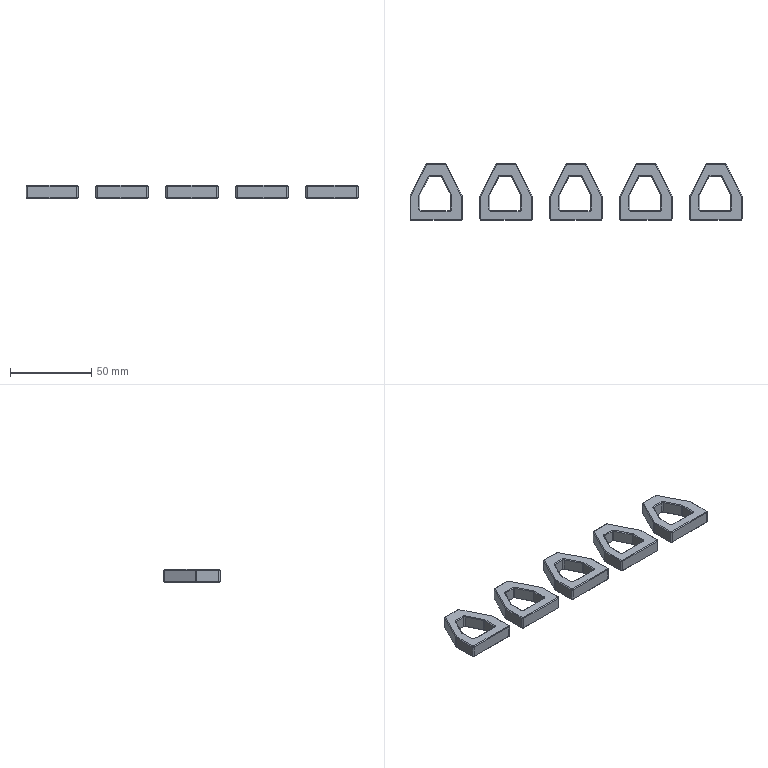NC program | NX | posted with a generic post | part box 204 x 35 x 8 mm
Lines 3701 to 4636 of 15564:
(ZLEVEL_PROFILE_COPY_1_COPY_1 , TOOL : D4)
N7382 T11 M6
N7384 G54
N7386 G17 G0 G90 X90.756 Y-9.215 S9500 M3
N7388 G43 Z30. H11
N7390 Z-0.385
N7392 G94 G1 X90.872 Y-9.415 F1000.
N7394 G3 X91.218 Y-9.615 R0.4
N7396 G1 X94.115 F1800.
N7398 Y-6.718
N7400 G3 X93.915 Y-6.372 R0.4
N7402 G1 X93.715 Y-6.256
N7404 G0 X90.641 Y-9.1 Z-0.769
N7406 G1 X90.757 Y-9.3 F1000.
N7408 G3 X91.103 Y-9.5 R0.4
N7410 G1 X94. F1800.
N7412 Y-6.603
N7414 G3 X93.8 Y-6.257 R0.4
N7416 G1 X93.6 Y-6.141
N7418 G0 X90.641 Y-9.1 Z-1.154
N7420 G1 X90.757 Y-9.3 F1000.
N7422 G3 X91.103 Y-9.5 R0.4
N7424 G1 X94. F1800.
N7426 Y-6.603
N7428 G3 X93.8 Y-6.257 R0.4
N7430 G1 X93.6 Y-6.141
N7432 G0 X90.641 Y-9.1 Z-1.538
N7434 G1 X90.757 Y-9.3 F1000.
N7436 G3 X91.103 Y-9.5 R0.4
N7438 G1 X94. F1800.
N7440 Y-6.603
N7442 G3 X93.8 Y-6.257 R0.4
N7444 G1 X93.6 Y-6.141
N7446 G0 X90.641 Y-9.1 Z-1.923
N7448 G1 X90.757 Y-9.3 F1000.
N7450 G3 X91.103 Y-9.5 R0.4
N7452 G1 X94. F1800.
N7454 Y-6.603
N7456 G3 X93.8 Y-6.257 R0.4
N7458 G1 X93.6 Y-6.141
N7460 G0 X90.641 Y-9.1 Z-2.308
N7462 G1 X90.757 Y-9.3 F1000.
N7464 G3 X91.103 Y-9.5 R0.4
N7466 G1 X94. F1800.
N7468 Y-6.603
N7470 G3 X93.8 Y-6.257 R0.4
N7472 G1 X93.6 Y-6.141
N7474 G0 X90.641 Y-9.1 Z-2.692
N7476 G1 X90.757 Y-9.3 F1000.
N7478 G3 X91.103 Y-9.5 R0.4
N7480 G1 X94. F1800.
N7482 Y-6.603
N7484 G3 X93.8 Y-6.257 R0.4
N7486 G1 X93.6 Y-6.141
N7488 G0 X90.641 Y-9.1 Z-3.077
N7490 G1 X90.757 Y-9.3 F1000.
N7492 G3 X91.103 Y-9.5 R0.4
N7494 G1 X94. F1800.
N7496 Y-6.603
N7498 G3 X93.8 Y-6.257 R0.4
N7500 G1 X93.6 Y-6.141
N7502 G0 X90.641 Y-9.1 Z-3.462
N7504 G1 X90.757 Y-9.3 F1000.
N7506 G3 X91.103 Y-9.5 R0.4
N7508 G1 X94. F1800.
N7510 Y-6.603
N7512 G3 X93.8 Y-6.257 R0.4
N7514 G1 X93.6 Y-6.141
N7516 G0 X90.641 Y-9.1 Z-3.846
N7518 G1 X90.757 Y-9.3 F1000.
N7520 G3 X91.103 Y-9.5 R0.4
N7522 G1 X94. F1800.
N7524 Y-6.603
N7526 G3 X93.8 Y-6.257 R0.4
N7528 G1 X93.6 Y-6.141
N7530 G0 X90.641 Y-9.1 Z-4.231
N7532 G1 X90.757 Y-9.3 F1000.
N7534 G3 X91.103 Y-9.5 R0.4
N7536 G1 X94. F1800.
N7538 Y-6.603
N7540 G3 X93.8 Y-6.257 R0.4
N7542 G1 X93.6 Y-6.141
N7544 G0 X90.641 Y-9.1 Z-4.615
N7546 G1 X90.757 Y-9.3 F1000.
N7548 G3 X91.103 Y-9.5 R0.4
N7550 G1 X94. F1800.
N7552 Y-6.603
N7554 G3 X93.8 Y-6.257 R0.4
N7556 G1 X93.6 Y-6.141
N7558 G0 X90.641 Y-9.1 Z-5.
N7560 G1 X90.757 Y-9.3 F1000.
N7562 G3 X91.103 Y-9.5 R0.4
N7564 G1 X94. F1800.
N7566 Y-6.603
N7568 G3 X93.8 Y-6.257 R0.4
N7570 G1 X93.6 Y-6.141
N7572 G0 X90.641 Y-9.1 Z-5.333
N7574 G1 X90.757 Y-9.3 F1000.
N7576 G3 X91.103 Y-9.5 R0.4
N7578 G1 X94. F1800.
N7580 Y-6.603
N7582 G3 X93.8 Y-6.257 R0.4
N7584 G1 X93.6 Y-6.141
N7586 G0 X90.641 Y-9.1 Z-5.667
N7588 G1 X90.757 Y-9.3 F1000.
N7590 G3 X91.103 Y-9.5 R0.4
N7592 G1 X94. F1800.
N7594 Y-6.603
N7596 G3 X93.8 Y-6.257 R0.4
N7598 G1 X93.6 Y-6.141
N7600 G0 X90.641 Y-9.1 Z-6.
N7602 G1 X90.757 Y-9.3 F1000.
N7604 G3 X91.103 Y-9.5 R0.4
N7606 G1 X94. F1800.
N7608 Y-6.603
N7610 G3 X93.8 Y-6.257 R0.4
N7612 G1 X93.6 Y-6.141
N7614 G0 X90.641 Y-9.1 Z-6.4
N7616 G1 X90.757 Y-9.3 F1000.
N7618 G3 X91.103 Y-9.5 R0.4
N7620 G1 X94. F1800.
N7622 Y-6.603
N7624 G3 X93.8 Y-6.257 R0.4
N7626 G1 X93.6 Y-6.141
N7628 G0 X90.641 Y-9.1 Z-6.8
N7630 G1 X90.757 Y-9.3 F1000.
N7632 G3 X91.103 Y-9.5 R0.4
N7634 G1 X94. F1800.
N7636 Y-6.603
N7638 G3 X93.8 Y-6.257 R0.4
N7640 G1 X93.6 Y-6.141
N7642 G0 X90.641 Y-9.1 Z-7.2
N7644 G1 X90.757 Y-9.3 F1000.
N7646 G3 X91.103 Y-9.5 R0.4
N7648 G1 X94. F1800.
N7650 Y-6.603
N7652 G3 X93.8 Y-6.257 R0.4
N7654 G1 X93.6 Y-6.141
N7656 G0 X90.641 Y-9.1 Z-7.6
N7658 G1 X90.757 Y-9.3 F1000.
N7660 G3 X91.103 Y-9.5 R0.4
N7662 G1 X94. F1800.
N7664 Y-6.603
N7666 G3 X93.8 Y-6.257 R0.4
N7668 G1 X93.6 Y-6.141
N7670 G0 X90.641 Y-9.1 Z-8.
N7672 G1 X90.757 Y-9.3 F1000.
N7674 G3 X91.103 Y-9.5 R0.4
N7676 G1 X94. F1800.
N7678 Y-6.603
N7680 G3 X93.8 Y-6.257 R0.4
N7682 G1 X93.6 Y-6.141
N7684 G0 Z30.
N7686 X93.715 Y-3.428
N7688 Z-0.385
N7690 G1 X93.915 Y-3.313 F1000.
N7692 G3 X94.115 Y-2.967 R0.4
N7694 G1 Y-2.361 F1800.
N7696 X93.845 Y-1.82
N7698 G3 X93.511 Y-1.6 R0.4
N7700 G1 X93.28 Y-1.586
N7702 G0 X93.6 Y-3.456 Z-0.769
N7704 G1 X93.8 Y-3.34 F1000.
N7706 G3 X94. Y-2.994 R0.4
N7708 G1 Y-2.389 F1800.
N7710 X93.729 Y-1.847
N7712 G3 X93.396 Y-1.627 R0.4
N7714 G1 X93.165 Y-1.613
N7716 G0 X93.6 Y-3.456 Z-1.154
N7718 G1 X93.8 Y-3.34 F1000.
N7720 G3 X94. Y-2.994 R0.4
N7722 G1 Y-2.389 F1800.
N7724 X93.729 Y-1.847
N7726 G3 X93.396 Y-1.627 R0.4
N7728 G1 X93.165 Y-1.613
N7730 G0 X93.6 Y-3.456 Z-1.538
N7732 G1 X93.8 Y-3.34 F1000.
N7734 G3 X94. Y-2.994 R0.4
N7736 G1 Y-2.389 F1800.
N7738 X93.729 Y-1.847
N7740 G3 X93.396 Y-1.627 R0.4
N7742 G1 X93.165 Y-1.613
N7744 G0 X93.6 Y-3.456 Z-1.923
N7746 G1 X93.8 Y-3.34 F1000.
N7748 G3 X94. Y-2.994 R0.4
N7750 G1 Y-2.389 F1800.
N7752 X93.729 Y-1.847
N7754 G3 X93.396 Y-1.627 R0.4
N7756 G1 X93.165 Y-1.613
N7758 G0 X93.6 Y-3.456 Z-2.308
N7760 G1 X93.8 Y-3.34 F1000.
N7762 G3 X94. Y-2.994 R0.4
N7764 G1 Y-2.389 F1800.
N7766 X93.729 Y-1.847
N7768 G3 X93.396 Y-1.627 R0.4
N7770 G1 X93.165 Y-1.613
N7772 G0 X93.6 Y-3.456 Z-2.692
N7774 G1 X93.8 Y-3.34 F1000.
N7776 G3 X94. Y-2.994 R0.4
N7778 G1 Y-2.389 F1800.
N7780 X93.729 Y-1.847
N7782 G3 X93.396 Y-1.627 R0.4
N7784 G1 X93.165 Y-1.613
N7786 G0 X93.6 Y-3.456 Z-3.077
N7788 G1 X93.8 Y-3.34 F1000.
N7790 G3 X94. Y-2.994 R0.4
N7792 G1 Y-2.389 F1800.
N7794 X93.729 Y-1.847
N7796 G3 X93.396 Y-1.627 R0.4
N7798 G1 X93.165 Y-1.613
N7800 G0 X93.6 Y-3.456 Z-3.462
N7802 G1 X93.8 Y-3.34 F1000.
N7804 G3 X94. Y-2.994 R0.4
N7806 G1 Y-2.389 F1800.
N7808 X93.729 Y-1.847
N7810 G3 X93.396 Y-1.627 R0.4
N7812 G1 X93.165 Y-1.613
N7814 G0 X93.6 Y-3.456 Z-3.846
N7816 G1 X93.8 Y-3.34 F1000.
N7818 G3 X94. Y-2.994 R0.4
N7820 G1 Y-2.389 F1800.
N7822 X93.729 Y-1.847
N7824 G3 X93.396 Y-1.627 R0.4
N7826 G1 X93.165 Y-1.613
N7828 G0 X93.6 Y-3.456 Z-4.231
N7830 G1 X93.8 Y-3.34 F1000.
N7832 G3 X94. Y-2.994 R0.4
N7834 G1 Y-2.389 F1800.
N7836 X93.729 Y-1.847
N7838 G3 X93.396 Y-1.627 R0.4
N7840 G1 X93.165 Y-1.613
N7842 G0 X93.6 Y-3.456 Z-4.615
N7844 G1 X93.8 Y-3.34 F1000.
N7846 G3 X94. Y-2.994 R0.4
N7848 G1 Y-2.389 F1800.
N7850 X93.729 Y-1.847
N7852 G3 X93.396 Y-1.627 R0.4
N7854 G1 X93.165 Y-1.613
N7856 G0 X93.6 Y-3.456 Z-5.
N7858 G1 X93.8 Y-3.34 F1000.
N7860 G3 X94. Y-2.994 R0.4
N7862 G1 Y-2.389 F1800.
N7864 X93.729 Y-1.847
N7866 G3 X93.396 Y-1.627 R0.4
N7868 G1 X93.165 Y-1.613
N7870 G0 X93.6 Y-3.456 Z-5.333
N7872 G1 X93.8 Y-3.34 F1000.
N7874 G3 X94. Y-2.994 R0.4
N7876 G1 Y-2.389 F1800.
N7878 X93.729 Y-1.847
N7880 G3 X93.396 Y-1.627 R0.4
N7882 G1 X93.165 Y-1.613
N7884 G0 X93.6 Y-3.456 Z-5.667
N7886 G1 X93.8 Y-3.34 F1000.
N7888 G3 X94. Y-2.994 R0.4
N7890 G1 Y-2.389 F1800.
N7892 X93.729 Y-1.847
N7894 G3 X93.396 Y-1.627 R0.4
N7896 G1 X93.165 Y-1.613
N7898 G0 X93.6 Y-3.456 Z-6.
N7900 G1 X93.8 Y-3.34 F1000.
N7902 G3 X94. Y-2.994 R0.4
N7904 G1 Y-2.389 F1800.
N7906 X93.729 Y-1.847
N7908 G3 X93.396 Y-1.627 R0.4
N7910 G1 X93.165 Y-1.613
N7912 G0 X93.6 Y-3.456 Z-6.4
N7914 G1 X93.8 Y-3.34 F1000.
N7916 G3 X94. Y-2.994 R0.4
N7918 G1 Y-2.389 F1800.
N7920 X93.729 Y-1.847
N7922 G3 X93.396 Y-1.627 R0.4
N7924 G1 X93.165 Y-1.613
N7926 G0 X93.6 Y-3.456 Z-6.8
N7928 G1 X93.8 Y-3.34 F1000.
N7930 G3 X94. Y-2.994 R0.4
N7932 G1 Y-2.389 F1800.
N7934 X93.729 Y-1.847
N7936 G3 X93.396 Y-1.627 R0.4
N7938 G1 X93.165 Y-1.613
N7940 G0 X93.6 Y-3.456 Z-7.2
N7942 G1 X93.8 Y-3.34 F1000.
N7944 G3 X94. Y-2.994 R0.4
N7946 G1 Y-2.389 F1800.
N7948 X93.729 Y-1.847
N7950 G3 X93.396 Y-1.627 R0.4
N7952 G1 X93.165 Y-1.613
N7954 G0 X93.6 Y-3.454 Z-7.6
N7956 G1 X93.8 Y-3.339 F1000.
N7958 G3 X94. Y-2.993 R0.4
N7960 G1 Y-2.389 F1800.
N7962 X93.73 Y-1.848
N7964 G3 X93.396 Y-1.628 R0.4
N7966 G1 X93.165 Y-1.614
N7968 G0 X93.6 Y-3.454 Z-8.
N7970 G1 X93.8 Y-3.339 F1000.
N7972 G3 X94. Y-2.993 R0.4
N7974 G1 Y-2.389 F1800.
N7976 X93.73 Y-1.848
N7978 G3 X93.396 Y-1.628 R0.4
N7980 G1 X93.165 Y-1.614
N7982 G0 Z30.
N7984 X89.759 Y5.457
N7986 Z-0.385
N7988 G1 X89.886 Y5.65 F1000.
N7990 G3 X89.91 Y6.049 R0.4
N7992 G1 X89.127 Y7.615 F1800.
N7994 X87.376
N7996 G3 X87.03 Y7.415 R0.4
N7998 G1 X86.914 Y7.215
N8000 G0 X89.688 Y5.342 Z-0.769
N8002 G1 X89.815 Y5.534 F1000.
N8004 G3 X89.839 Y5.934 R0.4
N8006 G1 X89.056 Y7.5 F1800.
N8008 X87.305
N8010 G3 X86.958 Y7.3 R0.4
N8012 G1 X86.843 Y7.1
N8014 G0 X89.688 Y5.342 Z-1.154
N8016 G1 X89.815 Y5.534 F1000.
N8018 G3 X89.839 Y5.934 R0.4
N8020 G1 X89.056 Y7.5 F1800.
N8022 X87.305
N8024 G3 X86.958 Y7.3 R0.4
N8026 G1 X86.843 Y7.1
N8028 G0 X89.688 Y5.342 Z-1.538
N8030 G1 X89.815 Y5.534 F1000.
N8032 G3 X89.839 Y5.934 R0.4
N8034 G1 X89.056 Y7.5 F1800.
N8036 X87.305
N8038 G3 X86.958 Y7.3 R0.4
N8040 G1 X86.843 Y7.1
N8042 G0 X89.688 Y5.342 Z-1.923
N8044 G1 X89.815 Y5.534 F1000.
N8046 G3 X89.839 Y5.934 R0.4
N8048 G1 X89.056 Y7.5 F1800.
N8050 X87.305
N8052 G3 X86.958 Y7.3 R0.4
N8054 G1 X86.843 Y7.1
N8056 G0 X89.688 Y5.342 Z-2.308
N8058 G1 X89.815 Y5.534 F1000.
N8060 G3 X89.839 Y5.934 R0.4
N8062 G1 X89.056 Y7.5 F1800.
N8064 X87.305
N8066 G3 X86.958 Y7.3 R0.4
N8068 G1 X86.843 Y7.1
N8070 G0 X89.688 Y5.342 Z-2.692
N8072 G1 X89.815 Y5.534 F1000.
N8074 G3 X89.839 Y5.934 R0.4
N8076 G1 X89.056 Y7.5 F1800.
N8078 X87.305
N8080 G3 X86.958 Y7.3 R0.4
N8082 G1 X86.843 Y7.1
N8084 G0 X89.688 Y5.342 Z-3.077
N8086 G1 X89.815 Y5.534 F1000.
N8088 G3 X89.839 Y5.934 R0.4
N8090 G1 X89.056 Y7.5 F1800.
N8092 X87.305
N8094 G3 X86.958 Y7.3 R0.4
N8096 G1 X86.843 Y7.1
N8098 G0 X89.688 Y5.342 Z-3.462
N8100 G1 X89.815 Y5.534 F1000.
N8102 G3 X89.839 Y5.934 R0.4
N8104 G1 X89.056 Y7.5 F1800.
N8106 X87.305
N8108 G3 X86.958 Y7.3 R0.4
N8110 G1 X86.843 Y7.1
N8112 G0 X89.688 Y5.342 Z-3.846
N8114 G1 X89.815 Y5.534 F1000.
N8116 G3 X89.839 Y5.934 R0.4
N8118 G1 X89.056 Y7.5 F1800.
N8120 X87.305
N8122 G3 X86.958 Y7.3 R0.4
N8124 G1 X86.843 Y7.1
N8126 G0 X89.688 Y5.342 Z-4.231
N8128 G1 X89.815 Y5.534 F1000.
N8130 G3 X89.839 Y5.934 R0.4
N8132 G1 X89.056 Y7.5 F1800.
N8134 X87.305
N8136 G3 X86.958 Y7.3 R0.4
N8138 G1 X86.843 Y7.1
N8140 G0 X89.688 Y5.342 Z-4.615
N8142 G1 X89.815 Y5.534 F1000.
N8144 G3 X89.839 Y5.934 R0.4
N8146 G1 X89.056 Y7.5 F1800.
N8148 X87.305
N8150 G3 X86.958 Y7.3 R0.4
N8152 G1 X86.843 Y7.1
N8154 G0 X89.688 Y5.342 Z-5.
N8156 G1 X89.815 Y5.534 F1000.
N8158 G3 X89.839 Y5.934 R0.4
N8160 G1 X89.056 Y7.5 F1800.
N8162 X87.305
N8164 G3 X86.958 Y7.3 R0.4
N8166 G1 X86.843 Y7.1
N8168 G0 X89.688 Y5.342 Z-5.333
N8170 G1 X89.815 Y5.534 F1000.
N8172 G3 X89.839 Y5.934 R0.4
N8174 G1 X89.056 Y7.5 F1800.
N8176 X87.305
N8178 G3 X86.958 Y7.3 R0.4
N8180 G1 X86.843 Y7.1
N8182 G0 X89.688 Y5.342 Z-5.667
N8184 G1 X89.815 Y5.534 F1000.
N8186 G3 X89.839 Y5.934 R0.4
N8188 G1 X89.056 Y7.5 F1800.
N8190 X87.305
N8192 G3 X86.958 Y7.3 R0.4
N8194 G1 X86.843 Y7.1
N8196 G0 X89.688 Y5.342 Z-6.
N8198 G1 X89.815 Y5.534 F1000.
N8200 G3 X89.839 Y5.934 R0.4
N8202 G1 X89.056 Y7.5 F1800.
N8204 X87.305
N8206 G3 X86.958 Y7.3 R0.4
N8208 G1 X86.843 Y7.1
N8210 G0 X89.688 Y5.342 Z-6.4
N8212 G1 X89.815 Y5.534 F1000.
N8214 G3 X89.839 Y5.934 R0.4
N8216 G1 X89.056 Y7.5 F1800.
N8218 X87.305
N8220 G3 X86.958 Y7.3 R0.4
N8222 G1 X86.843 Y7.1
N8224 G0 X89.688 Y5.342 Z-6.8
N8226 G1 X89.815 Y5.534 F1000.
N8228 G3 X89.839 Y5.934 R0.4
N8230 G1 X89.056 Y7.5 F1800.
N8232 X87.305
N8234 G3 X86.958 Y7.3 R0.4
N8236 G1 X86.843 Y7.1
N8238 G0 X89.688 Y5.342 Z-7.2
N8240 G1 X89.815 Y5.534 F1000.
N8242 G3 X89.839 Y5.934 R0.4
N8244 G1 X89.056 Y7.5 F1800.
N8246 X87.305
N8248 G3 X86.958 Y7.3 R0.4
N8250 G1 X86.843 Y7.1
N8252 G0 X89.686 Y5.344 Z-7.6
N8254 G1 X89.814 Y5.537 F1000.
N8256 G3 X89.838 Y5.936 R0.4
N8258 G1 X89.056 Y7.5 F1800.
N8260 X87.307
N8262 G3 X86.96 Y7.3 R0.4
N8264 G1 X86.845 Y7.1
N8266 G0 X89.686 Y5.344 Z-8.
N8268 G1 X89.814 Y5.537 F1000.
N8270 G3 X89.838 Y5.936 R0.4
N8272 G1 X89.056 Y7.5 F1800.
N8274 X87.307
N8276 G3 X86.96 Y7.3 R0.4
N8278 G1 X86.845 Y7.1
N8280 G0 Z30.
N8282 X86.086 Y7.215
N8284 Z-0.385
N8286 G1 X85.97 Y7.415 F1000.
N8288 G3 X85.624 Y7.615 R0.4
N8290 G1 X83.873 F1800.
N8292 X83.09 Y6.049
N8294 G3 X83.114 Y5.65 R0.4
N8296 G1 X83.241 Y5.457
N8298 G0 X86.157 Y7.1 Z-0.769
N8300 G1 X86.042 Y7.3 F1000.
N8302 G3 X85.695 Y7.5 R0.4
N8304 G1 X83.944 F1800.
N8306 X83.161 Y5.934
N8308 G3 X83.185 Y5.535 R0.4
N8310 G1 X83.313 Y5.342
N8312 G0 X86.157 Y7.1 Z-1.154
N8314 G1 X86.042 Y7.3 F1000.
N8316 G3 X85.695 Y7.5 R0.4
N8318 G1 X83.944 F1800.
N8320 X83.161 Y5.934
N8322 G3 X83.185 Y5.535 R0.4
N8324 G1 X83.313 Y5.342
N8326 G0 X86.157 Y7.1 Z-1.538
N8328 G1 X86.042 Y7.3 F1000.
N8330 G3 X85.695 Y7.5 R0.4
N8332 G1 X83.944 F1800.
N8334 X83.161 Y5.934
N8336 G3 X83.185 Y5.535 R0.4
N8338 G1 X83.313 Y5.342
N8340 G0 X86.157 Y7.1 Z-1.923
N8342 G1 X86.042 Y7.3 F1000.
N8344 G3 X85.695 Y7.5 R0.4
N8346 G1 X83.944 F1800.
N8348 X83.161 Y5.934
N8350 G3 X83.185 Y5.535 R0.4
N8352 G1 X83.313 Y5.342
N8354 G0 X86.157 Y7.1 Z-2.308
N8356 G1 X86.042 Y7.3 F1000.
N8358 G3 X85.695 Y7.5 R0.4
N8360 G1 X83.944 F1800.
N8362 X83.161 Y5.934
N8364 G3 X83.185 Y5.535 R0.4
N8366 G1 X83.313 Y5.342
N8368 G0 X86.157 Y7.1 Z-2.692
N8370 G1 X86.042 Y7.3 F1000.
N8372 G3 X85.695 Y7.5 R0.4
N8374 G1 X83.944 F1800.
N8376 X83.161 Y5.934
N8378 G3 X83.185 Y5.535 R0.4
N8380 G1 X83.313 Y5.342
N8382 G0 X86.157 Y7.1 Z-3.077
N8384 G1 X86.042 Y7.3 F1000.
N8386 G3 X85.695 Y7.5 R0.4
N8388 G1 X83.944 F1800.
N8390 X83.161 Y5.934
N8392 G3 X83.185 Y5.535 R0.4
N8394 G1 X83.313 Y5.342
N8396 G0 X86.157 Y7.1 Z-3.462
N8398 G1 X86.042 Y7.3 F1000.
N8400 G3 X85.695 Y7.5 R0.4
N8402 G1 X83.944 F1800.
N8404 X83.161 Y5.934
N8406 G3 X83.185 Y5.535 R0.4
N8408 G1 X83.313 Y5.342
N8410 G0 X86.157 Y7.1 Z-3.846
N8412 G1 X86.042 Y7.3 F1000.
N8414 G3 X85.695 Y7.5 R0.4
N8416 G1 X83.944 F1800.
N8418 X83.161 Y5.934
N8420 G3 X83.185 Y5.535 R0.4
N8422 G1 X83.313 Y5.342
N8424 G0 X86.157 Y7.1 Z-4.231
N8426 G1 X86.042 Y7.3 F1000.
N8428 G3 X85.695 Y7.5 R0.4
N8430 G1 X83.944 F1800.
N8432 X83.161 Y5.934
N8434 G3 X83.185 Y5.535 R0.4
N8436 G1 X83.313 Y5.342
N8438 G0 X86.157 Y7.1 Z-4.615
N8440 G1 X86.042 Y7.3 F1000.
N8442 G3 X85.695 Y7.5 R0.4
N8444 G1 X83.944 F1800.
N8446 X83.161 Y5.934
N8448 G3 X83.185 Y5.535 R0.4
N8450 G1 X83.313 Y5.342
N8452 G0 X86.157 Y7.1 Z-5.
N8454 G1 X86.042 Y7.3 F1000.
N8456 G3 X85.695 Y7.5 R0.4
N8458 G1 X83.944 F1800.
N8460 X83.161 Y5.934
N8462 G3 X83.185 Y5.535 R0.4
N8464 G1 X83.313 Y5.342
N8466 G0 X86.157 Y7.1 Z-5.333
N8468 G1 X86.042 Y7.3 F1000.
N8470 G3 X85.695 Y7.5 R0.4
N8472 G1 X83.944 F1800.
N8474 X83.161 Y5.934
N8476 G3 X83.185 Y5.535 R0.4
N8478 G1 X83.313 Y5.342
N8480 G0 X86.157 Y7.1 Z-5.667
N8482 G1 X86.042 Y7.3 F1000.
N8484 G3 X85.695 Y7.5 R0.4
N8486 G1 X83.944 F1800.
N8488 X83.161 Y5.934
N8490 G3 X83.185 Y5.535 R0.4
N8492 G1 X83.313 Y5.342
N8494 G0 X86.157 Y7.1 Z-6.
N8496 G1 X86.042 Y7.3 F1000.
N8498 G3 X85.695 Y7.5 R0.4
N8500 G1 X83.944 F1800.
N8502 X83.161 Y5.934
N8504 G3 X83.185 Y5.535 R0.4
N8506 G1 X83.313 Y5.342
N8508 G0 X86.157 Y7.1 Z-6.4
N8510 G1 X86.042 Y7.3 F1000.
N8512 G3 X85.695 Y7.5 R0.4
N8514 G1 X83.944 F1800.
N8516 X83.161 Y5.934
N8518 G3 X83.185 Y5.535 R0.4
N8520 G1 X83.313 Y5.342
N8522 G0 X86.157 Y7.1 Z-6.8
N8524 G1 X86.042 Y7.3 F1000.
N8526 G3 X85.695 Y7.5 R0.4
N8528 G1 X83.944 F1800.
N8530 X83.161 Y5.934
N8532 G3 X83.185 Y5.535 R0.4
N8534 G1 X83.313 Y5.342
N8536 G0 X86.157 Y7.1 Z-7.2
N8538 G1 X86.042 Y7.3 F1000.
N8540 G3 X85.695 Y7.5 R0.4
N8542 G1 X83.944 F1800.
N8544 X83.161 Y5.934
N8546 G3 X83.185 Y5.535 R0.4
N8548 G1 X83.313 Y5.342
N8550 G0 X86.157 Y7.1 Z-7.6
N8552 G1 X86.042 Y7.3 F1000.
N8554 G3 X85.695 Y7.5 R0.4
N8556 G1 X83.944 F1800.
N8558 X83.161 Y5.934
N8560 G3 X83.185 Y5.534 R0.4
N8562 G1 X83.312 Y5.342
N8564 G0 X86.157 Y7.1 Z-8.
N8566 G1 X86.042 Y7.3 F1000.
N8568 G3 X85.695 Y7.5 R0.4
N8570 G1 X83.944 F1800.
N8572 X83.161 Y5.934
N8574 G3 X83.185 Y5.534 R0.4
N8576 G1 X83.312 Y5.342
N8578 G0 Z30.
N8580 X79.72 Y-1.586
N8582 Z-0.385
N8584 G1 X79.489 Y-1.6 F1000.
N8586 G3 X79.155 Y-1.82 R0.4
N8588 G1 X78.885 Y-2.361 F1800.
N8590 Y-2.967
N8592 G3 X79.085 Y-3.313 R0.4
N8594 G1 X79.285 Y-3.428
N8596 G0 X79.835 Y-1.615 Z-0.769
N8598 G1 X79.604 Y-1.629 F1000.
N8600 G3 X79.27 Y-1.849 R0.4
N8602 G1 X79. Y-2.389 F1800.
N8604 Y-2.994
N8606 G3 X79.2 Y-3.34 R0.4
N8608 G1 X79.4 Y-3.456
N8610 G0 X79.835 Y-1.615 Z-1.154
N8612 G1 X79.604 Y-1.629 F1000.
N8614 G3 X79.27 Y-1.849 R0.4
N8616 G1 X79. Y-2.389 F1800.
N8618 Y-2.994
N8620 G3 X79.2 Y-3.34 R0.4
N8622 G1 X79.4 Y-3.456
N8624 G0 X79.835 Y-1.615 Z-1.538
N8626 G1 X79.604 Y-1.629 F1000.
N8628 G3 X79.27 Y-1.849 R0.4
N8630 G1 X79. Y-2.389 F1800.
N8632 Y-2.994
N8634 G3 X79.2 Y-3.34 R0.4
N8636 G1 X79.4 Y-3.456
N8638 G0 X79.835 Y-1.615 Z-1.923
N8640 G1 X79.604 Y-1.629 F1000.
N8642 G3 X79.27 Y-1.849 R0.4
N8644 G1 X79. Y-2.389 F1800.
N8646 Y-2.994
N8648 G3 X79.2 Y-3.34 R0.4
N8650 G1 X79.4 Y-3.456
N8652 G0 X79.835 Y-1.615 Z-2.308
N8654 G1 X79.604 Y-1.629 F1000.
N8656 G3 X79.27 Y-1.849 R0.4
N8658 G1 X79. Y-2.389 F1800.
N8660 Y-2.994
N8662 G3 X79.2 Y-3.34 R0.4
N8664 G1 X79.4 Y-3.456
N8666 G0 X79.835 Y-1.615 Z-2.692
N8668 G1 X79.604 Y-1.629 F1000.
N8670 G3 X79.27 Y-1.849 R0.4
N8672 G1 X79. Y-2.389 F1800.
N8674 Y-2.994
N8676 G3 X79.2 Y-3.34 R0.4
N8678 G1 X79.4 Y-3.456
N8680 G0 X79.835 Y-1.615 Z-3.077
N8682 G1 X79.604 Y-1.629 F1000.
N8684 G3 X79.27 Y-1.849 R0.4
N8686 G1 X79. Y-2.389 F1800.
N8688 Y-2.994
N8690 G3 X79.2 Y-3.34 R0.4
N8692 G1 X79.4 Y-3.456
N8694 G0 X79.835 Y-1.615 Z-3.462
N8696 G1 X79.604 Y-1.629 F1000.
N8698 G3 X79.27 Y-1.849 R0.4
N8700 G1 X79. Y-2.389 F1800.
N8702 Y-2.994
N8704 G3 X79.2 Y-3.34 R0.4
N8706 G1 X79.4 Y-3.456
N8708 G0 X79.835 Y-1.615 Z-3.846
N8710 G1 X79.604 Y-1.629 F1000.
N8712 G3 X79.27 Y-1.849 R0.4
N8714 G1 X79. Y-2.389 F1800.
N8716 Y-2.994
N8718 G3 X79.2 Y-3.34 R0.4
N8720 G1 X79.4 Y-3.456
N8722 G0 X79.835 Y-1.615 Z-4.231
N8724 G1 X79.604 Y-1.629 F1000.
N8726 G3 X79.27 Y-1.849 R0.4
N8728 G1 X79. Y-2.389 F1800.
N8730 Y-2.994
N8732 G3 X79.2 Y-3.34 R0.4
N8734 G1 X79.4 Y-3.456
N8736 G0 X79.835 Y-1.615 Z-4.615
N8738 G1 X79.604 Y-1.629 F1000.
N8740 G3 X79.27 Y-1.849 R0.4
N8742 G1 X79. Y-2.389 F1800.
N8744 Y-2.994
N8746 G3 X79.2 Y-3.34 R0.4
N8748 G1 X79.4 Y-3.456
N8750 G0 X79.835 Y-1.615 Z-5.
N8752 G1 X79.604 Y-1.629 F1000.
N8754 G3 X79.27 Y-1.849 R0.4
N8756 G1 X79. Y-2.389 F1800.
N8758 Y-2.994
N8760 G3 X79.2 Y-3.34 R0.4
N8762 G1 X79.4 Y-3.456
N8764 G0 X79.835 Y-1.615 Z-5.333
N8766 G1 X79.604 Y-1.629 F1000.
N8768 G3 X79.27 Y-1.849 R0.4
N8770 G1 X79. Y-2.389 F1800.
N8772 Y-2.994
N8774 G3 X79.2 Y-3.34 R0.4
N8776 G1 X79.4 Y-3.456
N8778 G0 X79.835 Y-1.615 Z-5.667
N8780 G1 X79.604 Y-1.629 F1000.
N8782 G3 X79.27 Y-1.849 R0.4
N8784 G1 X79. Y-2.389 F1800.
N8786 Y-2.994
N8788 G3 X79.2 Y-3.34 R0.4
N8790 G1 X79.4 Y-3.456
N8792 G0 X79.835 Y-1.615 Z-6.
N8794 G1 X79.604 Y-1.629 F1000.
N8796 G3 X79.27 Y-1.849 R0.4
N8798 G1 X79. Y-2.389 F1800.
N8800 Y-2.994
N8802 G3 X79.2 Y-3.34 R0.4
N8804 G1 X79.4 Y-3.456
N8806 G0 X79.835 Y-1.615 Z-6.4
N8808 G1 X79.604 Y-1.629 F1000.
N8810 G3 X79.27 Y-1.849 R0.4
N8812 G1 X79. Y-2.389 F1800.
N8814 Y-2.994
N8816 G3 X79.2 Y-3.34 R0.4
N8818 G1 X79.4 Y-3.456
N8820 G0 X79.835 Y-1.615 Z-6.8
N8822 G1 X79.604 Y-1.629 F1000.
N8824 G3 X79.27 Y-1.849 R0.4
N8826 G1 X79. Y-2.389 F1800.
N8828 Y-2.994
N8830 G3 X79.2 Y-3.34 R0.4
N8832 G1 X79.4 Y-3.456
N8834 G0 X79.835 Y-1.615 Z-7.2
N8836 G1 X79.604 Y-1.629 F1000.
N8838 G3 X79.27 Y-1.849 R0.4
N8840 G1 X79. Y-2.389 F1800.
N8842 Y-2.994
N8844 G3 X79.2 Y-3.34 R0.4
N8846 G1 X79.4 Y-3.456
N8848 G0 X79.826 Y-1.63 Z-7.6
N8850 G1 X79.596 Y-1.644 F1000.
N8852 G3 X79.262 Y-1.864 R0.4
N8854 G1 X79. Y-2.389 F1800.
N8856 Y-2.974
N8858 G3 X79.2 Y-3.321 R0.4
N8860 G1 X79.4 Y-3.436
N8862 G0 X79.826 Y-1.63 Z-8.
N8864 G1 X79.596 Y-1.644 F1000.
N8866 G3 X79.262 Y-1.864 R0.4
N8868 G1 X79. Y-2.389 F1800.
N8870 Y-2.974
N8872 G3 X79.2 Y-3.321 R0.4
N8874 G1 X79.4 Y-3.436
N8876 G0 Z30.
N8878 X79.285 Y-6.256
N8880 Z-0.385
N8882 G1 X79.085 Y-6.372 F1000.
N8884 G3 X78.885 Y-6.718 R0.4
N8886 G1 Y-9.615 F1800.
N8888 X81.782
N8890 G3 X82.128 Y-9.415 R0.4
N8892 G1 X82.244 Y-9.215
N8894 G0 X79.4 Y-6.141 Z-0.769
N8896 G1 X79.2 Y-6.257 F1000.
N8898 G3 X79. Y-6.603 R0.4
N8900 G1 Y-9.5 F1800.
N8902 X81.897
N8904 G3 X82.243 Y-9.3 R0.4
N8906 G1 X82.359 Y-9.1
N8908 G0 X79.4 Y-6.141 Z-1.154
N8910 G1 X79.2 Y-6.257 F1000.
N8912 G3 X79. Y-6.603 R0.4
N8914 G1 Y-9.5 F1800.
N8916 X81.897
N8918 G3 X82.243 Y-9.3 R0.4
N8920 G1 X82.359 Y-9.1
N8922 G0 X79.4 Y-6.141 Z-1.538
N8924 G1 X79.2 Y-6.257 F1000.
N8926 G3 X79. Y-6.603 R0.4
N8928 G1 Y-9.5 F1800.
N8930 X81.897
N8932 G3 X82.243 Y-9.3 R0.4
N8934 G1 X82.359 Y-9.1
N8936 G0 X79.4 Y-6.141 Z-1.923
N8938 G1 X79.2 Y-6.257 F1000.
N8940 G3 X79. Y-6.603 R0.4
N8942 G1 Y-9.5 F1800.
N8944 X81.897
N8946 G3 X82.243 Y-9.3 R0.4
N8948 G1 X82.359 Y-9.1
N8950 G0 X79.4 Y-6.141 Z-2.308
N8952 G1 X79.2 Y-6.257 F1000.
N8954 G3 X79. Y-6.603 R0.4
N8956 G1 Y-9.5 F1800.
N8958 X81.897
N8960 G3 X82.243 Y-9.3 R0.4
N8962 G1 X82.359 Y-9.1
N8964 G0 X79.4 Y-6.141 Z-2.692
N8966 G1 X79.2 Y-6.257 F1000.
N8968 G3 X79. Y-6.603 R0.4
N8970 G1 Y-9.5 F1800.
N8972 X81.897
N8974 G3 X82.243 Y-9.3 R0.4
N8976 G1 X82.359 Y-9.1
N8978 G0 X79.4 Y-6.141 Z-3.077
N8980 G1 X79.2 Y-6.257 F1000.
N8982 G3 X79. Y-6.603 R0.4
N8984 G1 Y-9.5 F1800.
N8986 X81.897
N8988 G3 X82.243 Y-9.3 R0.4
N8990 G1 X82.359 Y-9.1
N8992 G0 X79.4 Y-6.141 Z-3.462
N8994 G1 X79.2 Y-6.257 F1000.
N8996 G3 X79. Y-6.603 R0.4
N8998 G1 Y-9.5 F1800.
N9000 X81.897
N9002 G3 X82.243 Y-9.3 R0.4
N9004 G1 X82.359 Y-9.1
N9006 G0 X79.4 Y-6.141 Z-3.846
N9008 G1 X79.2 Y-6.257 F1000.
N9010 G3 X79. Y-6.603 R0.4
N9012 G1 Y-9.5 F1800.
N9014 X81.897
N9016 G3 X82.243 Y-9.3 R0.4
N9018 G1 X82.359 Y-9.1
N9020 G0 X79.4 Y-6.141 Z-4.231
N9022 G1 X79.2 Y-6.257 F1000.
N9024 G3 X79. Y-6.603 R0.4
N9026 G1 Y-9.5 F1800.
N9028 X81.897
N9030 G3 X82.243 Y-9.3 R0.4
N9032 G1 X82.359 Y-9.1
N9034 G0 X79.4 Y-6.141 Z-4.615
N9036 G1 X79.2 Y-6.257 F1000.
N9038 G3 X79. Y-6.603 R0.4
N9040 G1 Y-9.5 F1800.
N9042 X81.897
N9044 G3 X82.243 Y-9.3 R0.4
N9046 G1 X82.359 Y-9.1
N9048 G0 X79.4 Y-6.141 Z-5.
N9050 G1 X79.2 Y-6.257 F1000.
N9052 G3 X79. Y-6.603 R0.4
N9054 G1 Y-9.5 F1800.
N9056 X81.897
N9058 G3 X82.243 Y-9.3 R0.4
N9060 G1 X82.359 Y-9.1
N9062 G0 X79.4 Y-6.141 Z-5.333
N9064 G1 X79.2 Y-6.257 F1000.
N9066 G3 X79. Y-6.603 R0.4
N9068 G1 Y-9.5 F1800.
N9070 X81.897
N9072 G3 X82.243 Y-9.3 R0.4
N9074 G1 X82.359 Y-9.1
N9076 G0 X79.4 Y-6.141 Z-5.667
N9078 G1 X79.2 Y-6.257 F1000.
N9080 G3 X79. Y-6.603 R0.4
N9082 G1 Y-9.5 F1800.
N9084 X81.897
N9086 G3 X82.243 Y-9.3 R0.4
N9088 G1 X82.359 Y-9.1
N9090 G0 X79.4 Y-6.141 Z-6.
N9092 G1 X79.2 Y-6.257 F1000.
N9094 G3 X79. Y-6.603 R0.4
N9096 G1 Y-9.5 F1800.
N9098 X81.897
N9100 G3 X82.243 Y-9.3 R0.4
N9102 G1 X82.359 Y-9.1
N9104 G0 X79.4 Y-6.141 Z-6.4
N9106 G1 X79.2 Y-6.257 F1000.
N9108 G3 X79. Y-6.603 R0.4
N9110 G1 Y-9.5 F1800.
N9112 X81.897
N9114 G3 X82.243 Y-9.3 R0.4
N9116 G1 X82.359 Y-9.1
N9118 G0 X79.4 Y-6.141 Z-6.8
N9120 G1 X79.2 Y-6.257 F1000.
N9122 G3 X79. Y-6.603 R0.4
N9124 G1 Y-9.5 F1800.
N9126 X81.897
N9128 G3 X82.243 Y-9.3 R0.4
N9130 G1 X82.359 Y-9.1
N9132 G0 X79.4 Y-6.141 Z-7.2
N9134 G1 X79.2 Y-6.257 F1000.
N9136 G3 X79. Y-6.603 R0.4
N9138 G1 Y-9.5 F1800.
N9140 X81.897
N9142 G3 X82.243 Y-9.3 R0.4
N9144 G1 X82.359 Y-9.1
N9146 G0 X79.4 Y-6.141 Z-7.6
N9148 G1 X79.2 Y-6.257 F1000.
N9150 G3 X79. Y-6.603 R0.4
N9152 G1 Y-9.5 F1800.
N9154 X81.897
N9156 G3 X82.243 Y-9.3 R0.4
N9158 G1 X82.359 Y-9.1
N9160 G0 X79.4 Y-6.141 Z-8.
N9162 G1 X79.2 Y-6.257 F1000.
N9164 G3 X79. Y-6.603 R0.4
N9166 G1 Y-9.5 F1800.
N9168 X81.897
N9170 G3 X82.243 Y-9.3 R0.4
N9172 G1 X82.359 Y-9.1
N9174 G0 Z30.
N9176 X47.756 Y-9.215
N9178 Z-0.385
N9180 G1 X47.872 Y-9.415 F1000.
N9182 G3 X48.218 Y-9.615 R0.4
N9184 G1 X51.115 F1800.
N9186 Y-6.718
N9188 G3 X50.915 Y-6.372 R0.4
N9190 G1 X50.715 Y-6.256
N9192 G0 X47.641 Y-9.1 Z-0.769
N9194 G1 X47.757 Y-9.3 F1000.
N9196 G3 X48.103 Y-9.5 R0.4
N9198 G1 X51. F1800.
N9200 Y-6.603
N9202 G3 X50.8 Y-6.257 R0.4
N9204 G1 X50.6 Y-6.141
N9206 G0 X47.641 Y-9.1 Z-1.154
N9208 G1 X47.757 Y-9.3 F1000.
N9210 G3 X48.103 Y-9.5 R0.4
N9212 G1 X51. F1800.
N9214 Y-6.603
N9216 G3 X50.8 Y-6.257 R0.4
N9218 G1 X50.6 Y-6.141
N9220 G0 X47.641 Y-9.1 Z-1.538
N9222 G1 X47.757 Y-9.3 F1000.
N9224 G3 X48.103 Y-9.5 R0.4
N9226 G1 X51. F1800.
N9228 Y-6.603
N9230 G3 X50.8 Y-6.257 R0.4
N9232 G1 X50.6 Y-6.141
N9234 G0 X47.641 Y-9.1 Z-1.923
N9236 G1 X47.757 Y-9.3 F1000.
N9238 G3 X48.103 Y-9.5 R0.4
N9240 G1 X51. F1800.
N9242 Y-6.603
N9244 G3 X50.8 Y-6.257 R0.4
N9246 G1 X50.6 Y-6.141